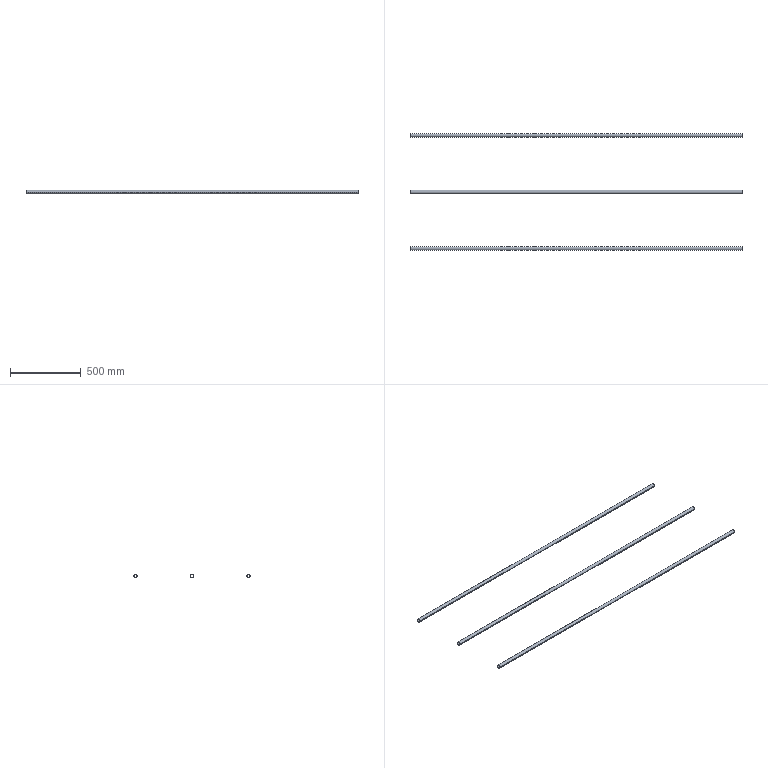Part | STEP file | E3-中转釜护栏4栏杆_Default<As Machined> | 3 solids | 18 faces | box 2348 x 825 x 25 mm | volume 780061 mm3 | cylinder 12 | plane 6 | commonest cylinder face diameters 22 x6 25 x6
STEP:
#1=CARTESIAN_POINT('',(0.,0.,0.));
#2=DIRECTION('',(0.,0.,1.));
#3=DIRECTION('',(1.,0.,0.));
#4=AXIS2_PLACEMENT_3D('',#1,#2,#3);
#5=CARTESIAN_POINT('',(1174.,787.5,0.));
#6=VERTEX_POINT('',#5);
#7=CARTESIAN_POINT('',(1174.,812.5,0.));
#8=VERTEX_POINT('',#7);
#9=CARTESIAN_POINT('',(1174.,800.,0.));
#10=DIRECTION('',(-1.,0.,0.));
#11=DIRECTION('',(0.,1.,0.));
#12=AXIS2_PLACEMENT_3D('',#9,#10,#11);
#13=CIRCLE('',#12,12.5);
#14=CARTESIAN_POINT('',(1174.,800.,0.));
#15=DIRECTION('',(-1.,0.,0.));
#16=DIRECTION('',(0.,-1.,0.));
#17=AXIS2_PLACEMENT_3D('',#14,#15,#16);
#18=CYLINDRICAL_SURFACE('',#17,12.5);
#19=CARTESIAN_POINT('',(-3.142,0.));
#20=DIRECTION('',(1.,0.));
#21=VECTOR('',#20,1.);
#22=LINE('',#19,#21);
#23=(GEOMETRIC_REPRESENTATION_CONTEXT(2)PARAMETRIC_REPRESENTATION_CONTEXT()REPRESENTATION_CONTEXT('',''));
#24=DEFINITIONAL_REPRESENTATION('',(#22),#23);
#25=PCURVE('',#18,#24);
#26=CARTESIAN_POINT('',(1174.,800.,0.));
#27=DIRECTION('',(1.,0.,0.));
#28=DIRECTION('',(0.,1.,0.));
#29=AXIS2_PLACEMENT_3D('',#26,#27,#28);
#30=PLANE('',#29);
#31=CARTESIAN_POINT('',(12.5,0.));
#32=CARTESIAN_POINT('',(12.5,-21.651));
#33=CARTESIAN_POINT('',(-6.25,-10.825));
#34=CARTESIAN_POINT('',(-25.,0.));
#35=CARTESIAN_POINT('',(-6.25,10.825));
#36=CARTESIAN_POINT('',(12.5,21.651));
#37=CARTESIAN_POINT('',(12.5,0.));
#38=(BOUNDED_CURVE()B_SPLINE_CURVE(2,(#31,#32,#33,#34,#35,#36,#37),.UNSPECIFIED.,.T.,.F.)B_SPLINE_CURVE_WITH_KNOTS((1,2,2,2,2,1),(-2.094,0.,2.094,4.189,6.283,8.378),.UNSPECIFIED.)CURVE()GEOMETRIC_REPRESENTATION_ITEM()RATIONAL_B_SPLINE_CURVE((1.,0.5,1.,0.5,1.,0.5,1.))REPRESENTATION_ITEM(''));
#39=(GEOMETRIC_REPRESENTATION_CONTEXT(2)PARAMETRIC_REPRESENTATION_CONTEXT()REPRESENTATION_CONTEXT('',''));
#40=DEFINITIONAL_REPRESENTATION('',(#38),#39);
#41=PCURVE('',#30,#40);
#42=SURFACE_CURVE('',#13,(#25,#41),.PCURVE_S1.);
#43=EDGE_CURVE('',#6,#8,#42,.T.);
#44=ORIENTED_EDGE('',*,*,#43,.T.);
#45=CARTESIAN_POINT('',(-1174.,812.5,0.));
#46=VERTEX_POINT('',#45);
#47=CARTESIAN_POINT('',(1174.,812.5,0.));
#48=DIRECTION('',(-1.,0.,0.));
#49=VECTOR('',#48,1.);
#50=LINE('',#47,#49);
#51=CARTESIAN_POINT('',(3.142,0.));
#52=DIRECTION('',(0.,1.));
#53=VECTOR('',#52,1.);
#54=LINE('',#51,#53);
#55=(GEOMETRIC_REPRESENTATION_CONTEXT(2)PARAMETRIC_REPRESENTATION_CONTEXT()REPRESENTATION_CONTEXT('',''));
#56=DEFINITIONAL_REPRESENTATION('',(#54),#55);
#57=PCURVE('',#18,#56);
#58=CARTESIAN_POINT('',(1174.,800.,0.));
#59=DIRECTION('',(-1.,0.,0.));
#60=DIRECTION('',(0.,-1.,0.));
#61=AXIS2_PLACEMENT_3D('',#58,#59,#60);
#62=CYLINDRICAL_SURFACE('',#61,12.5);
#63=CARTESIAN_POINT('',(3.142,0.));
#64=DIRECTION('',(0.,1.));
#65=VECTOR('',#64,1.);
#66=LINE('',#63,#65);
#67=(GEOMETRIC_REPRESENTATION_CONTEXT(2)PARAMETRIC_REPRESENTATION_CONTEXT()REPRESENTATION_CONTEXT('',''));
#68=DEFINITIONAL_REPRESENTATION('',(#66),#67);
#69=PCURVE('',#62,#68);
#70=SURFACE_CURVE('',#50,(#57,#69),.PCURVE_S1.);
#71=EDGE_CURVE('',#8,#46,#70,.T.);
#72=ORIENTED_EDGE('',*,*,#71,.T.);
#73=CARTESIAN_POINT('',(-1174.,787.5,0.));
#74=VERTEX_POINT('',#73);
#75=CARTESIAN_POINT('',(-1174.,800.,0.));
#76=DIRECTION('',(-1.,0.,0.));
#77=DIRECTION('',(0.,1.,0.));
#78=AXIS2_PLACEMENT_3D('',#75,#76,#77);
#79=CIRCLE('',#78,12.5);
#80=CARTESIAN_POINT('',(-3.142,2348.));
#81=DIRECTION('',(1.,0.));
#82=VECTOR('',#81,1.);
#83=LINE('',#80,#82);
#84=(GEOMETRIC_REPRESENTATION_CONTEXT(2)PARAMETRIC_REPRESENTATION_CONTEXT()REPRESENTATION_CONTEXT('',''));
#85=DEFINITIONAL_REPRESENTATION('',(#83),#84);
#86=PCURVE('',#18,#85);
#87=CARTESIAN_POINT('',(-1174.,800.,0.));
#88=DIRECTION('',(1.,0.,0.));
#89=DIRECTION('',(0.,1.,0.));
#90=AXIS2_PLACEMENT_3D('',#87,#88,#89);
#91=PLANE('',#90);
#92=CARTESIAN_POINT('',(12.5,0.));
#93=CARTESIAN_POINT('',(12.5,-21.651));
#94=CARTESIAN_POINT('',(-6.25,-10.825));
#95=CARTESIAN_POINT('',(-25.,0.));
#96=CARTESIAN_POINT('',(-6.25,10.825));
#97=CARTESIAN_POINT('',(12.5,21.651));
#98=CARTESIAN_POINT('',(12.5,0.));
#99=(BOUNDED_CURVE()B_SPLINE_CURVE(2,(#92,#93,#94,#95,#96,#97,#98),.UNSPECIFIED.,.T.,.F.)B_SPLINE_CURVE_WITH_KNOTS((1,2,2,2,2,1),(-2.094,0.,2.094,4.189,6.283,8.378),.UNSPECIFIED.)CURVE()GEOMETRIC_REPRESENTATION_ITEM()RATIONAL_B_SPLINE_CURVE((1.,0.5,1.,0.5,1.,0.5,1.))REPRESENTATION_ITEM(''));
#100=(GEOMETRIC_REPRESENTATION_CONTEXT(2)PARAMETRIC_REPRESENTATION_CONTEXT()REPRESENTATION_CONTEXT('',''));
#101=DEFINITIONAL_REPRESENTATION('',(#99),#100);
#102=PCURVE('',#91,#101);
#103=SURFACE_CURVE('',#79,(#86,#102),.PCURVE_S1.);
#104=EDGE_CURVE('',#74,#46,#103,.T.);
#105=ORIENTED_EDGE('',*,*,#104,.F.);
#106=CARTESIAN_POINT('',(1174.,787.5,0.));
#107=DIRECTION('',(-1.,0.,0.));
#108=VECTOR('',#107,1.);
#109=LINE('',#106,#108);
#110=CARTESIAN_POINT('',(0.,0.));
#111=DIRECTION('',(0.,1.));
#112=VECTOR('',#111,1.);
#113=LINE('',#110,#112);
#114=(GEOMETRIC_REPRESENTATION_CONTEXT(2)PARAMETRIC_REPRESENTATION_CONTEXT()REPRESENTATION_CONTEXT('',''));
#115=DEFINITIONAL_REPRESENTATION('',(#113),#114);
#116=PCURVE('',#18,#115);
#117=CARTESIAN_POINT('',(6.283,0.));
#118=DIRECTION('',(0.,1.));
#119=VECTOR('',#118,1.);
#120=LINE('',#117,#119);
#121=(GEOMETRIC_REPRESENTATION_CONTEXT(2)PARAMETRIC_REPRESENTATION_CONTEXT()REPRESENTATION_CONTEXT('',''));
#122=DEFINITIONAL_REPRESENTATION('',(#120),#121);
#123=PCURVE('',#62,#122);
#124=SURFACE_CURVE('',#109,(#116,#123),.PCURVE_S1.);
#125=EDGE_CURVE('',#6,#74,#124,.T.);
#126=ORIENTED_EDGE('',*,*,#125,.F.);
#127=EDGE_LOOP('',(#44,#72,#105,#126));
#128=FACE_BOUND('',#127,.T.);
#129=ADVANCED_FACE('',(#128),#18,.T.);
#130=CARTESIAN_POINT('',(1174.,789.,0.));
#131=VERTEX_POINT('',#130);
#132=CARTESIAN_POINT('',(-1174.,789.,0.));
#133=VERTEX_POINT('',#132);
#134=CARTESIAN_POINT('',(1174.,789.,0.));
#135=DIRECTION('',(-1.,0.,0.));
#136=VECTOR('',#135,1.);
#137=LINE('',#134,#136);
#138=CARTESIAN_POINT('',(1174.,800.,0.));
#139=DIRECTION('',(-1.,0.,0.));
#140=DIRECTION('',(0.,-1.,0.));
#141=AXIS2_PLACEMENT_3D('',#138,#139,#140);
#142=CYLINDRICAL_SURFACE('',#141,11.);
#143=CARTESIAN_POINT('',(6.283,0.));
#144=DIRECTION('',(0.,1.));
#145=VECTOR('',#144,1.);
#146=LINE('',#143,#145);
#147=(GEOMETRIC_REPRESENTATION_CONTEXT(2)PARAMETRIC_REPRESENTATION_CONTEXT()REPRESENTATION_CONTEXT('',''));
#148=DEFINITIONAL_REPRESENTATION('',(#146),#147);
#149=PCURVE('',#142,#148);
#150=CARTESIAN_POINT('',(1174.,800.,0.));
#151=DIRECTION('',(-1.,0.,0.));
#152=DIRECTION('',(0.,-1.,0.));
#153=AXIS2_PLACEMENT_3D('',#150,#151,#152);
#154=CYLINDRICAL_SURFACE('',#153,11.);
#155=CARTESIAN_POINT('',(0.,0.));
#156=DIRECTION('',(0.,1.));
#157=VECTOR('',#156,1.);
#158=LINE('',#155,#157);
#159=(GEOMETRIC_REPRESENTATION_CONTEXT(2)PARAMETRIC_REPRESENTATION_CONTEXT()REPRESENTATION_CONTEXT('',''));
#160=DEFINITIONAL_REPRESENTATION('',(#158),#159);
#161=PCURVE('',#154,#160);
#162=SURFACE_CURVE('',#137,(#149,#161),.PCURVE_S1.);
#163=EDGE_CURVE('',#131,#133,#162,.T.);
#164=ORIENTED_EDGE('',*,*,#163,.T.);
#165=CARTESIAN_POINT('',(-1174.,811.,0.));
#166=VERTEX_POINT('',#165);
#167=CARTESIAN_POINT('',(-1174.,800.,0.));
#168=DIRECTION('',(-1.,0.,0.));
#169=DIRECTION('',(0.,1.,0.));
#170=AXIS2_PLACEMENT_3D('',#167,#168,#169);
#171=CIRCLE('',#170,11.);
#172=CARTESIAN_POINT('',(3.142,2348.));
#173=DIRECTION('',(1.,0.));
#174=VECTOR('',#173,1.);
#175=LINE('',#172,#174);
#176=(GEOMETRIC_REPRESENTATION_CONTEXT(2)PARAMETRIC_REPRESENTATION_CONTEXT()REPRESENTATION_CONTEXT('',''));
#177=DEFINITIONAL_REPRESENTATION('',(#175),#176);
#178=PCURVE('',#142,#177);
#179=CARTESIAN_POINT('',(11.,0.));
#180=CARTESIAN_POINT('',(11.,-19.053));
#181=CARTESIAN_POINT('',(-5.5,-9.526));
#182=CARTESIAN_POINT('',(-22.,0.));
#183=CARTESIAN_POINT('',(-5.5,9.526));
#184=CARTESIAN_POINT('',(11.,19.053));
#185=CARTESIAN_POINT('',(11.,0.));
#186=(BOUNDED_CURVE()B_SPLINE_CURVE(2,(#179,#180,#181,#182,#183,#184,#185),.UNSPECIFIED.,.T.,.F.)B_SPLINE_CURVE_WITH_KNOTS((1,2,2,2,2,1),(-2.094,0.,2.094,4.189,6.283,8.378),.UNSPECIFIED.)CURVE()GEOMETRIC_REPRESENTATION_ITEM()RATIONAL_B_SPLINE_CURVE((1.,0.5,1.,0.5,1.,0.5,1.))REPRESENTATION_ITEM(''));
#187=(GEOMETRIC_REPRESENTATION_CONTEXT(2)PARAMETRIC_REPRESENTATION_CONTEXT()REPRESENTATION_CONTEXT('',''));
#188=DEFINITIONAL_REPRESENTATION('',(#186),#187);
#189=PCURVE('',#91,#188);
#190=SURFACE_CURVE('',#171,(#178,#189),.PCURVE_S1.);
#191=EDGE_CURVE('',#166,#133,#190,.T.);
#192=ORIENTED_EDGE('',*,*,#191,.F.);
#193=CARTESIAN_POINT('',(1174.,811.,0.));
#194=VERTEX_POINT('',#193);
#195=CARTESIAN_POINT('',(1174.,811.,0.));
#196=DIRECTION('',(-1.,0.,0.));
#197=VECTOR('',#196,1.);
#198=LINE('',#195,#197);
#199=CARTESIAN_POINT('',(3.142,0.));
#200=DIRECTION('',(0.,1.));
#201=VECTOR('',#200,1.);
#202=LINE('',#199,#201);
#203=(GEOMETRIC_REPRESENTATION_CONTEXT(2)PARAMETRIC_REPRESENTATION_CONTEXT()REPRESENTATION_CONTEXT('',''));
#204=DEFINITIONAL_REPRESENTATION('',(#202),#203);
#205=PCURVE('',#142,#204);
#206=CARTESIAN_POINT('',(3.142,0.));
#207=DIRECTION('',(0.,1.));
#208=VECTOR('',#207,1.);
#209=LINE('',#206,#208);
#210=(GEOMETRIC_REPRESENTATION_CONTEXT(2)PARAMETRIC_REPRESENTATION_CONTEXT()REPRESENTATION_CONTEXT('',''));
#211=DEFINITIONAL_REPRESENTATION('',(#209),#210);
#212=PCURVE('',#154,#211);
#213=SURFACE_CURVE('',#198,(#205,#212),.PCURVE_S1.);
#214=EDGE_CURVE('',#194,#166,#213,.T.);
#215=ORIENTED_EDGE('',*,*,#214,.F.);
#216=CARTESIAN_POINT('',(1174.,800.,0.));
#217=DIRECTION('',(-1.,0.,0.));
#218=DIRECTION('',(0.,1.,0.));
#219=AXIS2_PLACEMENT_3D('',#216,#217,#218);
#220=CIRCLE('',#219,11.);
#221=CARTESIAN_POINT('',(3.142,0.));
#222=DIRECTION('',(1.,0.));
#223=VECTOR('',#222,1.);
#224=LINE('',#221,#223);
#225=(GEOMETRIC_REPRESENTATION_CONTEXT(2)PARAMETRIC_REPRESENTATION_CONTEXT()REPRESENTATION_CONTEXT('',''));
#226=DEFINITIONAL_REPRESENTATION('',(#224),#225);
#227=PCURVE('',#142,#226);
#228=CARTESIAN_POINT('',(11.,0.));
#229=CARTESIAN_POINT('',(11.,-19.053));
#230=CARTESIAN_POINT('',(-5.5,-9.526));
#231=CARTESIAN_POINT('',(-22.,0.));
#232=CARTESIAN_POINT('',(-5.5,9.526));
#233=CARTESIAN_POINT('',(11.,19.053));
#234=CARTESIAN_POINT('',(11.,0.));
#235=(BOUNDED_CURVE()B_SPLINE_CURVE(2,(#228,#229,#230,#231,#232,#233,#234),.UNSPECIFIED.,.T.,.F.)B_SPLINE_CURVE_WITH_KNOTS((1,2,2,2,2,1),(-2.094,0.,2.094,4.189,6.283,8.378),.UNSPECIFIED.)CURVE()GEOMETRIC_REPRESENTATION_ITEM()RATIONAL_B_SPLINE_CURVE((1.,0.5,1.,0.5,1.,0.5,1.))REPRESENTATION_ITEM(''));
#236=(GEOMETRIC_REPRESENTATION_CONTEXT(2)PARAMETRIC_REPRESENTATION_CONTEXT()REPRESENTATION_CONTEXT('',''));
#237=DEFINITIONAL_REPRESENTATION('',(#235),#236);
#238=PCURVE('',#30,#237);
#239=SURFACE_CURVE('',#220,(#227,#238),.PCURVE_S1.);
#240=EDGE_CURVE('',#194,#131,#239,.T.);
#241=ORIENTED_EDGE('',*,*,#240,.T.);
#242=EDGE_LOOP('',(#164,#192,#215,#241));
#243=FACE_BOUND('',#242,.F.);
#244=ADVANCED_FACE('',(#243),#142,.F.);
#245=CARTESIAN_POINT('',(-1174.,800.,0.));
#246=DIRECTION('',(-1.,0.,0.));
#247=DIRECTION('',(0.,1.,0.));
#248=AXIS2_PLACEMENT_3D('',#245,#246,#247);
#249=CIRCLE('',#248,11.);
#250=CARTESIAN_POINT('',(-3.142,2348.));
#251=DIRECTION('',(1.,0.));
#252=VECTOR('',#251,1.);
#253=LINE('',#250,#252);
#254=(GEOMETRIC_REPRESENTATION_CONTEXT(2)PARAMETRIC_REPRESENTATION_CONTEXT()REPRESENTATION_CONTEXT('',''));
#255=DEFINITIONAL_REPRESENTATION('',(#253),#254);
#256=PCURVE('',#154,#255);
#257=CARTESIAN_POINT('',(11.,0.));
#258=CARTESIAN_POINT('',(11.,-19.053));
#259=CARTESIAN_POINT('',(-5.5,-9.526));
#260=CARTESIAN_POINT('',(-22.,0.));
#261=CARTESIAN_POINT('',(-5.5,9.526));
#262=CARTESIAN_POINT('',(11.,19.053));
#263=CARTESIAN_POINT('',(11.,0.));
#264=(BOUNDED_CURVE()B_SPLINE_CURVE(2,(#257,#258,#259,#260,#261,#262,#263),.UNSPECIFIED.,.T.,.F.)B_SPLINE_CURVE_WITH_KNOTS((1,2,2,2,2,1),(-2.094,0.,2.094,4.189,6.283,8.378),.UNSPECIFIED.)CURVE()GEOMETRIC_REPRESENTATION_ITEM()RATIONAL_B_SPLINE_CURVE((1.,0.5,1.,0.5,1.,0.5,1.))REPRESENTATION_ITEM(''));
#265=(GEOMETRIC_REPRESENTATION_CONTEXT(2)PARAMETRIC_REPRESENTATION_CONTEXT()REPRESENTATION_CONTEXT('',''));
#266=DEFINITIONAL_REPRESENTATION('',(#264),#265);
#267=PCURVE('',#91,#266);
#268=SURFACE_CURVE('',#249,(#256,#267),.PCURVE_S1.);
#269=EDGE_CURVE('',#133,#166,#268,.T.);
#270=ORIENTED_EDGE('',*,*,#269,.F.);
#271=ORIENTED_EDGE('',*,*,#163,.F.);
#272=CARTESIAN_POINT('',(1174.,800.,0.));
#273=DIRECTION('',(-1.,0.,0.));
#274=DIRECTION('',(0.,1.,0.));
#275=AXIS2_PLACEMENT_3D('',#272,#273,#274);
#276=CIRCLE('',#275,11.);
#277=CARTESIAN_POINT('',(-3.142,0.));
#278=DIRECTION('',(1.,0.));
#279=VECTOR('',#278,1.);
#280=LINE('',#277,#279);
#281=(GEOMETRIC_REPRESENTATION_CONTEXT(2)PARAMETRIC_REPRESENTATION_CONTEXT()REPRESENTATION_CONTEXT('',''));
#282=DEFINITIONAL_REPRESENTATION('',(#280),#281);
#283=PCURVE('',#154,#282);
#284=CARTESIAN_POINT('',(11.,0.));
#285=CARTESIAN_POINT('',(11.,-19.053));
#286=CARTESIAN_POINT('',(-5.5,-9.526));
#287=CARTESIAN_POINT('',(-22.,0.));
#288=CARTESIAN_POINT('',(-5.5,9.526));
#289=CARTESIAN_POINT('',(11.,19.053));
#290=CARTESIAN_POINT('',(11.,0.));
#291=(BOUNDED_CURVE()B_SPLINE_CURVE(2,(#284,#285,#286,#287,#288,#289,#290),.UNSPECIFIED.,.T.,.F.)B_SPLINE_CURVE_WITH_KNOTS((1,2,2,2,2,1),(-2.094,0.,2.094,4.189,6.283,8.378),.UNSPECIFIED.)CURVE()GEOMETRIC_REPRESENTATION_ITEM()RATIONAL_B_SPLINE_CURVE((1.,0.5,1.,0.5,1.,0.5,1.))REPRESENTATION_ITEM(''));
#292=(GEOMETRIC_REPRESENTATION_CONTEXT(2)PARAMETRIC_REPRESENTATION_CONTEXT()REPRESENTATION_CONTEXT('',''));
#293=DEFINITIONAL_REPRESENTATION('',(#291),#292);
#294=PCURVE('',#30,#293);
#295=SURFACE_CURVE('',#276,(#283,#294),.PCURVE_S1.);
#296=EDGE_CURVE('',#131,#194,#295,.T.);
#297=ORIENTED_EDGE('',*,*,#296,.T.);
#298=ORIENTED_EDGE('',*,*,#214,.T.);
#299=EDGE_LOOP('',(#270,#271,#297,#298));
#300=FACE_BOUND('',#299,.F.);
#301=ADVANCED_FACE('',(#300),#154,.F.);
#302=ORIENTED_EDGE('',*,*,#71,.F.);
#303=CARTESIAN_POINT('',(1174.,800.,0.));
#304=DIRECTION('',(-1.,0.,0.));
#305=DIRECTION('',(0.,1.,0.));
#306=AXIS2_PLACEMENT_3D('',#303,#304,#305);
#307=CIRCLE('',#306,12.5);
#308=CARTESIAN_POINT('',(3.142,0.));
#309=DIRECTION('',(1.,0.));
#310=VECTOR('',#309,1.);
#311=LINE('',#308,#310);
#312=(GEOMETRIC_REPRESENTATION_CONTEXT(2)PARAMETRIC_REPRESENTATION_CONTEXT()REPRESENTATION_CONTEXT('',''));
#313=DEFINITIONAL_REPRESENTATION('',(#311),#312);
#314=PCURVE('',#62,#313);
#315=CARTESIAN_POINT('',(12.5,0.));
#316=CARTESIAN_POINT('',(12.5,-21.651));
#317=CARTESIAN_POINT('',(-6.25,-10.825));
#318=CARTESIAN_POINT('',(-25.,0.));
#319=CARTESIAN_POINT('',(-6.25,10.825));
#320=CARTESIAN_POINT('',(12.5,21.651));
#321=CARTESIAN_POINT('',(12.5,0.));
#322=(BOUNDED_CURVE()B_SPLINE_CURVE(2,(#315,#316,#317,#318,#319,#320,#321),.UNSPECIFIED.,.T.,.F.)B_SPLINE_CURVE_WITH_KNOTS((1,2,2,2,2,1),(-2.094,0.,2.094,4.189,6.283,8.378),.UNSPECIFIED.)CURVE()GEOMETRIC_REPRESENTATION_ITEM()RATIONAL_B_SPLINE_CURVE((1.,0.5,1.,0.5,1.,0.5,1.))REPRESENTATION_ITEM(''));
#323=(GEOMETRIC_REPRESENTATION_CONTEXT(2)PARAMETRIC_REPRESENTATION_CONTEXT()REPRESENTATION_CONTEXT('',''));
#324=DEFINITIONAL_REPRESENTATION('',(#322),#323);
#325=PCURVE('',#30,#324);
#326=SURFACE_CURVE('',#307,(#314,#325),.PCURVE_S1.);
#327=EDGE_CURVE('',#8,#6,#326,.T.);
#328=ORIENTED_EDGE('',*,*,#327,.T.);
#329=ORIENTED_EDGE('',*,*,#125,.T.);
#330=CARTESIAN_POINT('',(-1174.,800.,0.));
#331=DIRECTION('',(-1.,0.,0.));
#332=DIRECTION('',(0.,1.,0.));
#333=AXIS2_PLACEMENT_3D('',#330,#331,#332);
#334=CIRCLE('',#333,12.5);
#335=CARTESIAN_POINT('',(3.142,2348.));
#336=DIRECTION('',(1.,0.));
#337=VECTOR('',#336,1.);
#338=LINE('',#335,#337);
#339=(GEOMETRIC_REPRESENTATION_CONTEXT(2)PARAMETRIC_REPRESENTATION_CONTEXT()REPRESENTATION_CONTEXT('',''));
#340=DEFINITIONAL_REPRESENTATION('',(#338),#339);
#341=PCURVE('',#62,#340);
#342=CARTESIAN_POINT('',(12.5,0.));
#343=CARTESIAN_POINT('',(12.5,-21.651));
#344=CARTESIAN_POINT('',(-6.25,-10.825));
#345=CARTESIAN_POINT('',(-25.,0.));
#346=CARTESIAN_POINT('',(-6.25,10.825));
#347=CARTESIAN_POINT('',(12.5,21.651));
#348=CARTESIAN_POINT('',(12.5,0.));
#349=(BOUNDED_CURVE()B_SPLINE_CURVE(2,(#342,#343,#344,#345,#346,#347,#348),.UNSPECIFIED.,.T.,.F.)B_SPLINE_CURVE_WITH_KNOTS((1,2,2,2,2,1),(-2.094,0.,2.094,4.189,6.283,8.378),.UNSPECIFIED.)CURVE()GEOMETRIC_REPRESENTATION_ITEM()RATIONAL_B_SPLINE_CURVE((1.,0.5,1.,0.5,1.,0.5,1.))REPRESENTATION_ITEM(''));
#350=(GEOMETRIC_REPRESENTATION_CONTEXT(2)PARAMETRIC_REPRESENTATION_CONTEXT()REPRESENTATION_CONTEXT('',''));
#351=DEFINITIONAL_REPRESENTATION('',(#349),#350);
#352=PCURVE('',#91,#351);
#353=SURFACE_CURVE('',#334,(#341,#352),.PCURVE_S1.);
#354=EDGE_CURVE('',#46,#74,#353,.T.);
#355=ORIENTED_EDGE('',*,*,#354,.F.);
#356=EDGE_LOOP('',(#302,#328,#329,#355));
#357=FACE_BOUND('',#356,.T.);
#358=ADVANCED_FACE('',(#357),#62,.T.);
#359=ORIENTED_EDGE('',*,*,#296,.T.);
#360=ORIENTED_EDGE('',*,*,#240,.T.);
#361=EDGE_LOOP('',(#359,#360));
#362=FACE_BOUND('',#361,.T.);
#363=ORIENTED_EDGE('',*,*,#43,.F.);
#364=ORIENTED_EDGE('',*,*,#327,.F.);
#365=EDGE_LOOP('',(#363,#364));
#366=FACE_BOUND('',#365,.T.);
#367=ADVANCED_FACE('',(#362,#366),#30,.T.);
#368=ORIENTED_EDGE('',*,*,#269,.F.);
#369=ORIENTED_EDGE('',*,*,#191,.F.);
#370=EDGE_LOOP('',(#368,#369));
#371=FACE_BOUND('',#370,.T.);
#372=ORIENTED_EDGE('',*,*,#104,.T.);
#373=ORIENTED_EDGE('',*,*,#354,.T.);
#374=EDGE_LOOP('',(#372,#373));
#375=FACE_BOUND('',#374,.T.);
#376=ADVANCED_FACE('',(#371,#375),#91,.F.);
#377=CLOSED_SHELL('',(#129,#244,#301,#358,#367,#376));
#378=MANIFOLD_SOLID_BREP('',#377);
#379=CARTESIAN_POINT('',(1174.,-12.5,0.));
#380=VERTEX_POINT('',#379);
#381=CARTESIAN_POINT('',(1174.,12.5,0.));
#382=VERTEX_POINT('',#381);
#383=CARTESIAN_POINT('',(1174.,0.,0.));
#384=DIRECTION('',(-1.,0.,0.));
#385=DIRECTION('',(0.,1.,0.));
#386=AXIS2_PLACEMENT_3D('',#383,#384,#385);
#387=CIRCLE('',#386,12.5);
#388=CARTESIAN_POINT('',(1174.,0.,0.));
#389=DIRECTION('',(-1.,0.,0.));
#390=DIRECTION('',(0.,-1.,0.));
#391=AXIS2_PLACEMENT_3D('',#388,#389,#390);
#392=CYLINDRICAL_SURFACE('',#391,12.5);
#393=CARTESIAN_POINT('',(-3.142,0.));
#394=DIRECTION('',(1.,0.));
#395=VECTOR('',#394,1.);
#396=LINE('',#393,#395);
#397=(GEOMETRIC_REPRESENTATION_CONTEXT(2)PARAMETRIC_REPRESENTATION_CONTEXT()REPRESENTATION_CONTEXT('',''));
#398=DEFINITIONAL_REPRESENTATION('',(#396),#397);
#399=PCURVE('',#392,#398);
#400=CARTESIAN_POINT('',(1174.,0.,0.));
#401=DIRECTION('',(1.,0.,0.));
#402=DIRECTION('',(0.,1.,0.));
#403=AXIS2_PLACEMENT_3D('',#400,#401,#402);
#404=PLANE('',#403);
#405=CARTESIAN_POINT('',(12.5,0.));
#406=CARTESIAN_POINT('',(12.5,-21.651));
#407=CARTESIAN_POINT('',(-6.25,-10.825));
#408=CARTESIAN_POINT('',(-25.,0.));
#409=CARTESIAN_POINT('',(-6.25,10.825));
#410=CARTESIAN_POINT('',(12.5,21.651));
#411=CARTESIAN_POINT('',(12.5,0.));
#412=(BOUNDED_CURVE()B_SPLINE_CURVE(2,(#405,#406,#407,#408,#409,#410,#411),.UNSPECIFIED.,.T.,.F.)B_SPLINE_CURVE_WITH_KNOTS((1,2,2,2,2,1),(-2.094,0.,2.094,4.189,6.283,8.378),.UNSPECIFIED.)CURVE()GEOMETRIC_REPRESENTATION_ITEM()RATIONAL_B_SPLINE_CURVE((1.,0.5,1.,0.5,1.,0.5,1.))REPRESENTATION_ITEM(''));
#413=(GEOMETRIC_REPRESENTATION_CONTEXT(2)PARAMETRIC_REPRESENTATION_CONTEXT()REPRESENTATION_CONTEXT('',''));
#414=DEFINITIONAL_REPRESENTATION('',(#412),#413);
#415=PCURVE('',#404,#414);
#416=SURFACE_CURVE('',#387,(#399,#415),.PCURVE_S1.);
#417=EDGE_CURVE('',#380,#382,#416,.T.);
#418=ORIENTED_EDGE('',*,*,#417,.T.);
#419=CARTESIAN_POINT('',(-1174.,12.5,0.));
#420=VERTEX_POINT('',#419);
#421=CARTESIAN_POINT('',(1174.,12.5,0.));
#422=DIRECTION('',(-1.,0.,0.));
#423=VECTOR('',#422,1.);
#424=LINE('',#421,#423);
#425=CARTESIAN_POINT('',(3.142,0.));
#426=DIRECTION('',(0.,1.));
#427=VECTOR('',#426,1.);
#428=LINE('',#425,#427);
#429=(GEOMETRIC_REPRESENTATION_CONTEXT(2)PARAMETRIC_REPRESENTATION_CONTEXT()REPRESENTATION_CONTEXT('',''));
#430=DEFINITIONAL_REPRESENTATION('',(#428),#429);
#431=PCURVE('',#392,#430);
#432=CARTESIAN_POINT('',(1174.,0.,0.));
#433=DIRECTION('',(-1.,0.,0.));
#434=DIRECTION('',(0.,-1.,0.));
#435=AXIS2_PLACEMENT_3D('',#432,#433,#434);
#436=CYLINDRICAL_SURFACE('',#435,12.5);
#437=CARTESIAN_POINT('',(3.142,0.));
#438=DIRECTION('',(0.,1.));
#439=VECTOR('',#438,1.);
#440=LINE('',#437,#439);
#441=(GEOMETRIC_REPRESENTATION_CONTEXT(2)PARAMETRIC_REPRESENTATION_CONTEXT()REPRESENTATION_CONTEXT('',''));
#442=DEFINITIONAL_REPRESENTATION('',(#440),#441);
#443=PCURVE('',#436,#442);
#444=SURFACE_CURVE('',#424,(#431,#443),.PCURVE_S1.);
#445=EDGE_CURVE('',#382,#420,#444,.T.);
#446=ORIENTED_EDGE('',*,*,#445,.T.);
#447=CARTESIAN_POINT('',(-1174.,-12.5,0.));
#448=VERTEX_POINT('',#447);
#449=CARTESIAN_POINT('',(-1174.,0.,0.));
#450=DIRECTION('',(-1.,0.,0.));
#451=DIRECTION('',(0.,1.,0.));
#452=AXIS2_PLACEMENT_3D('',#449,#450,#451);
#453=CIRCLE('',#452,12.5);
#454=CARTESIAN_POINT('',(-3.142,2348.));
#455=DIRECTION('',(1.,0.));
#456=VECTOR('',#455,1.);
#457=LINE('',#454,#456);
#458=(GEOMETRIC_REPRESENTATION_CONTEXT(2)PARAMETRIC_REPRESENTATION_CONTEXT()REPRESENTATION_CONTEXT('',''));
#459=DEFINITIONAL_REPRESENTATION('',(#457),#458);
#460=PCURVE('',#392,#459);
#461=CARTESIAN_POINT('',(-1174.,0.,0.));
#462=DIRECTION('',(1.,0.,0.));
#463=DIRECTION('',(0.,1.,0.));
#464=AXIS2_PLACEMENT_3D('',#461,#462,#463);
#465=PLANE('',#464);
#466=CARTESIAN_POINT('',(12.5,0.));
#467=CARTESIAN_POINT('',(12.5,-21.651));
#468=CARTESIAN_POINT('',(-6.25,-10.825));
#469=CARTESIAN_POINT('',(-25.,0.));
#470=CARTESIAN_POINT('',(-6.25,10.825));
#471=CARTESIAN_POINT('',(12.5,21.651));
#472=CARTESIAN_POINT('',(12.5,0.));
#473=(BOUNDED_CURVE()B_SPLINE_CURVE(2,(#466,#467,#468,#469,#470,#471,#472),.UNSPECIFIED.,.T.,.F.)B_SPLINE_CURVE_WITH_KNOTS((1,2,2,2,2,1),(-2.094,0.,2.094,4.189,6.283,8.378),.UNSPECIFIED.)CURVE()GEOMETRIC_REPRESENTATION_ITEM()RATIONAL_B_SPLINE_CURVE((1.,0.5,1.,0.5,1.,0.5,1.))REPRESENTATION_ITEM(''));
#474=(GEOMETRIC_REPRESENTATION_CONTEXT(2)PARAMETRIC_REPRESENTATION_CONTEXT()REPRESENTATION_CONTEXT('',''));
#475=DEFINITIONAL_REPRESENTATION('',(#473),#474);
#476=PCURVE('',#465,#475);
#477=SURFACE_CURVE('',#453,(#460,#476),.PCURVE_S1.);
#478=EDGE_CURVE('',#448,#420,#477,.T.);
#479=ORIENTED_EDGE('',*,*,#478,.F.);
#480=CARTESIAN_POINT('',(1174.,-12.5,0.));
#481=DIRECTION('',(-1.,0.,0.));
#482=VECTOR('',#481,1.);
#483=LINE('',#480,#482);
#484=CARTESIAN_POINT('',(0.,0.));
#485=DIRECTION('',(0.,1.));
#486=VECTOR('',#485,1.);
#487=LINE('',#484,#486);
#488=(GEOMETRIC_REPRESENTATION_CONTEXT(2)PARAMETRIC_REPRESENTATION_CONTEXT()REPRESENTATION_CONTEXT('',''));
#489=DEFINITIONAL_REPRESENTATION('',(#487),#488);
#490=PCURVE('',#392,#489);
#491=CARTESIAN_POINT('',(6.283,0.));
#492=DIRECTION('',(0.,1.));
#493=VECTOR('',#492,1.);
#494=LINE('',#491,#493);
#495=(GEOMETRIC_REPRESENTATION_CONTEXT(2)PARAMETRIC_REPRESENTATION_CONTEXT()REPRESENTATION_CONTEXT('',''));
#496=DEFINITIONAL_REPRESENTATION('',(#494),#495);
#497=PCURVE('',#436,#496);
#498=SURFACE_CURVE('',#483,(#490,#497),.PCURVE_S1.);
#499=EDGE_CURVE('',#380,#448,#498,.T.);
#500=ORIENTED_EDGE('',*,*,#499,.F.);
#501=EDGE_LOOP('',(#418,#446,#479,#500));
#502=FACE_BOUND('',#501,.T.);
#503=ADVANCED_FACE('',(#502),#392,.T.);
#504=CARTESIAN_POINT('',(1174.,-11.,0.));
#505=VERTEX_POINT('',#504);
#506=CARTESIAN_POINT('',(-1174.,-11.,0.));
#507=VERTEX_POINT('',#506);
#508=CARTESIAN_POINT('',(1174.,-11.,0.));
#509=DIRECTION('',(-1.,0.,0.));
#510=VECTOR('',#509,1.);
#511=LINE('',#508,#510);
#512=CARTESIAN_POINT('',(1174.,0.,0.));
#513=DIRECTION('',(-1.,0.,0.));
#514=DIRECTION('',(0.,-1.,0.));
#515=AXIS2_PLACEMENT_3D('',#512,#513,#514);
#516=CYLINDRICAL_SURFACE('',#515,11.);
#517=CARTESIAN_POINT('',(6.283,0.));
#518=DIRECTION('',(0.,1.));
#519=VECTOR('',#518,1.);
#520=LINE('',#517,#519);
#521=(GEOMETRIC_REPRESENTATION_CONTEXT(2)PARAMETRIC_REPRESENTATION_CONTEXT()REPRESENTATION_CONTEXT('',''));
#522=DEFINITIONAL_REPRESENTATION('',(#520),#521);
#523=PCURVE('',#516,#522);
#524=CARTESIAN_POINT('',(1174.,0.,0.));
#525=DIRECTION('',(-1.,0.,0.));
#526=DIRECTION('',(0.,-1.,0.));
#527=AXIS2_PLACEMENT_3D('',#524,#525,#526);
#528=CYLINDRICAL_SURFACE('',#527,11.);
#529=CARTESIAN_POINT('',(0.,0.));
#530=DIRECTION('',(0.,1.));
#531=VECTOR('',#530,1.);
#532=LINE('',#529,#531);
#533=(GEOMETRIC_REPRESENTATION_CONTEXT(2)PARAMETRIC_REPRESENTATION_CONTEXT()REPRESENTATION_CONTEXT('',''));
#534=DEFINITIONAL_REPRESENTATION('',(#532),#533);
#535=PCURVE('',#528,#534);
#536=SURFACE_CURVE('',#511,(#523,#535),.PCURVE_S1.);
#537=EDGE_CURVE('',#505,#507,#536,.T.);
#538=ORIENTED_EDGE('',*,*,#537,.T.);
#539=CARTESIAN_POINT('',(-1174.,11.,0.));
#540=VERTEX_POINT('',#539);
#541=CARTESIAN_POINT('',(-1174.,0.,0.));
#542=DIRECTION('',(-1.,0.,0.));
#543=DIRECTION('',(0.,1.,0.));
#544=AXIS2_PLACEMENT_3D('',#541,#542,#543);
#545=CIRCLE('',#544,11.);
#546=CARTESIAN_POINT('',(3.142,2348.));
#547=DIRECTION('',(1.,0.));
#548=VECTOR('',#547,1.);
#549=LINE('',#546,#548);
#550=(GEOMETRIC_REPRESENTATION_CONTEXT(2)PARAMETRIC_REPRESENTATION_CONTEXT()REPRESENTATION_CONTEXT('',''));
#551=DEFINITIONAL_REPRESENTATION('',(#549),#550);
#552=PCURVE('',#516,#551);
#553=CARTESIAN_POINT('',(11.,0.));
#554=CARTESIAN_POINT('',(11.,-19.053));
#555=CARTESIAN_POINT('',(-5.5,-9.526));
#556=CARTESIAN_POINT('',(-22.,0.));
#557=CARTESIAN_POINT('',(-5.5,9.526));
#558=CARTESIAN_POINT('',(11.,19.053));
#559=CARTESIAN_POINT('',(11.,0.));
#560=(BOUNDED_CURVE()B_SPLINE_CURVE(2,(#553,#554,#555,#556,#557,#558,#559),.UNSPECIFIED.,.T.,.F.)B_SPLINE_CURVE_WITH_KNOTS((1,2,2,2,2,1),(-2.094,0.,2.094,4.189,6.283,8.378),.UNSPECIFIED.)CURVE()GEOMETRIC_REPRESENTATION_ITEM()RATIONAL_B_SPLINE_CURVE((1.,0.5,1.,0.5,1.,0.5,1.))REPRESENTATION_ITEM(''));
#561=(GEOMETRIC_REPRESENTATION_CONTEXT(2)PARAMETRIC_REPRESENTATION_CONTEXT()REPRESENTATION_CONTEXT('',''));
#562=DEFINITIONAL_REPRESENTATION('',(#560),#561);
#563=PCURVE('',#465,#562);
#564=SURFACE_CURVE('',#545,(#552,#563),.PCURVE_S1.);
#565=EDGE_CURVE('',#540,#507,#564,.T.);
#566=ORIENTED_EDGE('',*,*,#565,.F.);
#567=CARTESIAN_POINT('',(1174.,11.,0.));
#568=VERTEX_POINT('',#567);
#569=CARTESIAN_POINT('',(1174.,11.,0.));
#570=DIRECTION('',(-1.,0.,0.));
#571=VECTOR('',#570,1.);
#572=LINE('',#569,#571);
#573=CARTESIAN_POINT('',(3.142,0.));
#574=DIRECTION('',(0.,1.));
#575=VECTOR('',#574,1.);
#576=LINE('',#573,#575);
#577=(GEOMETRIC_REPRESENTATION_CONTEXT(2)PARAMETRIC_REPRESENTATION_CONTEXT()REPRESENTATION_CONTEXT('',''));
#578=DEFINITIONAL_REPRESENTATION('',(#576),#577);
#579=PCURVE('',#516,#578);
#580=CARTESIAN_POINT('',(3.142,0.));
#581=DIRECTION('',(0.,1.));
#582=VECTOR('',#581,1.);
#583=LINE('',#580,#582);
#584=(GEOMETRIC_REPRESENTATION_CONTEXT(2)PARAMETRIC_REPRESENTATION_CONTEXT()REPRESENTATION_CONTEXT('',''));
#585=DEFINITIONAL_REPRESENTATION('',(#583),#584);
#586=PCURVE('',#528,#585);
#587=SURFACE_CURVE('',#572,(#579,#586),.PCURVE_S1.);
#588=EDGE_CURVE('',#568,#540,#587,.T.);
#589=ORIENTED_EDGE('',*,*,#588,.F.);
#590=CARTESIAN_POINT('',(1174.,0.,0.));
#591=DIRECTION('',(-1.,0.,0.));
#592=DIRECTION('',(0.,1.,0.));
#593=AXIS2_PLACEMENT_3D('',#590,#591,#592);
#594=CIRCLE('',#593,11.);
#595=CARTESIAN_POINT('',(3.142,0.));
#596=DIRECTION('',(1.,0.));
#597=VECTOR('',#596,1.);
#598=LINE('',#595,#597);
#599=(GEOMETRIC_REPRESENTATION_CONTEXT(2)PARAMETRIC_REPRESENTATION_CONTEXT()REPRESENTATION_CONTEXT('',''));
#600=DEFINITIONAL_REPRESENTATION('',(#598),#599);
#601=PCURVE('',#516,#600);
#602=CARTESIAN_POINT('',(11.,0.));
#603=CARTESIAN_POINT('',(11.,-19.053));
#604=CARTESIAN_POINT('',(-5.5,-9.526));
#605=CARTESIAN_POINT('',(-22.,0.));
#606=CARTESIAN_POINT('',(-5.5,9.526));
#607=CARTESIAN_POINT('',(11.,19.053));
#608=CARTESIAN_POINT('',(11.,0.));
#609=(BOUNDED_CURVE()B_SPLINE_CURVE(2,(#602,#603,#604,#605,#606,#607,#608),.UNSPECIFIED.,.T.,.F.)B_SPLINE_CURVE_WITH_KNOTS((1,2,2,2,2,1),(-2.094,0.,2.094,4.189,6.283,8.378),.UNSPECIFIED.)CURVE()GEOMETRIC_REPRESENTATION_ITEM()RATIONAL_B_SPLINE_CURVE((1.,0.5,1.,0.5,1.,0.5,1.))REPRESENTATION_ITEM(''));
#610=(GEOMETRIC_REPRESENTATION_CONTEXT(2)PARAMETRIC_REPRESENTATION_CONTEXT()REPRESENTATION_CONTEXT('',''));
#611=DEFINITIONAL_REPRESENTATION('',(#609),#610);
#612=PCURVE('',#404,#611);
#613=SURFACE_CURVE('',#594,(#601,#612),.PCURVE_S1.);
#614=EDGE_CURVE('',#568,#505,#613,.T.);
#615=ORIENTED_EDGE('',*,*,#614,.T.);
#616=EDGE_LOOP('',(#538,#566,#589,#615));
#617=FACE_BOUND('',#616,.F.);
#618=ADVANCED_FACE('',(#617),#516,.F.);
#619=CARTESIAN_POINT('',(-1174.,0.,0.));
#620=DIRECTION('',(-1.,0.,0.));
#621=DIRECTION('',(0.,1.,0.));
#622=AXIS2_PLACEMENT_3D('',#619,#620,#621);
#623=CIRCLE('',#622,11.);
#624=CARTESIAN_POINT('',(-3.142,2348.));
#625=DIRECTION('',(1.,0.));
#626=VECTOR('',#625,1.);
#627=LINE('',#624,#626);
#628=(GEOMETRIC_REPRESENTATION_CONTEXT(2)PARAMETRIC_REPRESENTATION_CONTEXT()REPRESENTATION_CONTEXT('',''));
#629=DEFINITIONAL_REPRESENTATION('',(#627),#628);
#630=PCURVE('',#528,#629);
#631=CARTESIAN_POINT('',(11.,0.));
#632=CARTESIAN_POINT('',(11.,-19.053));
#633=CARTESIAN_POINT('',(-5.5,-9.526));
#634=CARTESIAN_POINT('',(-22.,0.));
#635=CARTESIAN_POINT('',(-5.5,9.526));
#636=CARTESIAN_POINT('',(11.,19.053));
#637=CARTESIAN_POINT('',(11.,0.));
#638=(BOUNDED_CURVE()B_SPLINE_CURVE(2,(#631,#632,#633,#634,#635,#636,#637),.UNSPECIFIED.,.T.,.F.)B_SPLINE_CURVE_WITH_KNOTS((1,2,2,2,2,1),(-2.094,0.,2.094,4.189,6.283,8.378),.UNSPECIFIED.)CURVE()GEOMETRIC_REPRESENTATION_ITEM()RATIONAL_B_SPLINE_CURVE((1.,0.5,1.,0.5,1.,0.5,1.))REPRESENTATION_ITEM(''));
#639=(GEOMETRIC_REPRESENTATION_CONTEXT(2)PARAMETRIC_REPRESENTATION_CONTEXT()REPRESENTATION_CONTEXT('',''));
#640=DEFINITIONAL_REPRESENTATION('',(#638),#639);
#641=PCURVE('',#465,#640);
#642=SURFACE_CURVE('',#623,(#630,#641),.PCURVE_S1.);
#643=EDGE_CURVE('',#507,#540,#642,.T.);
#644=ORIENTED_EDGE('',*,*,#643,.F.);
#645=ORIENTED_EDGE('',*,*,#537,.F.);
#646=CARTESIAN_POINT('',(1174.,0.,0.));
#647=DIRECTION('',(-1.,0.,0.));
#648=DIRECTION('',(0.,1.,0.));
#649=AXIS2_PLACEMENT_3D('',#646,#647,#648);
#650=CIRCLE('',#649,11.);
#651=CARTESIAN_POINT('',(-3.142,0.));
#652=DIRECTION('',(1.,0.));
#653=VECTOR('',#652,1.);
#654=LINE('',#651,#653);
#655=(GEOMETRIC_REPRESENTATION_CONTEXT(2)PARAMETRIC_REPRESENTATION_CONTEXT()REPRESENTATION_CONTEXT('',''));
#656=DEFINITIONAL_REPRESENTATION('',(#654),#655);
#657=PCURVE('',#528,#656);
#658=CARTESIAN_POINT('',(11.,0.));
#659=CARTESIAN_POINT('',(11.,-19.053));
#660=CARTESIAN_POINT('',(-5.5,-9.526));
#661=CARTESIAN_POINT('',(-22.,0.));
#662=CARTESIAN_POINT('',(-5.5,9.526));
#663=CARTESIAN_POINT('',(11.,19.053));
#664=CARTESIAN_POINT('',(11.,0.));
#665=(BOUNDED_CURVE()B_SPLINE_CURVE(2,(#658,#659,#660,#661,#662,#663,#664),.UNSPECIFIED.,.T.,.F.)B_SPLINE_CURVE_WITH_KNOTS((1,2,2,2,2,1),(-2.094,0.,2.094,4.189,6.283,8.378),.UNSPECIFIED.)CURVE()GEOMETRIC_REPRESENTATION_ITEM()RATIONAL_B_SPLINE_CURVE((1.,0.5,1.,0.5,1.,0.5,1.))REPRESENTATION_ITEM(''));
#666=(GEOMETRIC_REPRESENTATION_CONTEXT(2)PARAMETRIC_REPRESENTATION_CONTEXT()REPRESENTATION_CONTEXT('',''));
#667=DEFINITIONAL_REPRESENTATION('',(#665),#666);
#668=PCURVE('',#404,#667);
#669=SURFACE_CURVE('',#650,(#657,#668),.PCURVE_S1.);
#670=EDGE_CURVE('',#505,#568,#669,.T.);
#671=ORIENTED_EDGE('',*,*,#670,.T.);
#672=ORIENTED_EDGE('',*,*,#588,.T.);
#673=EDGE_LOOP('',(#644,#645,#671,#672));
#674=FACE_BOUND('',#673,.F.);
#675=ADVANCED_FACE('',(#674),#528,.F.);
#676=ORIENTED_EDGE('',*,*,#445,.F.);
#677=CARTESIAN_POINT('',(1174.,0.,0.));
#678=DIRECTION('',(-1.,0.,0.));
#679=DIRECTION('',(0.,1.,0.));
#680=AXIS2_PLACEMENT_3D('',#677,#678,#679);
#681=CIRCLE('',#680,12.5);
#682=CARTESIAN_POINT('',(3.142,0.));
#683=DIRECTION('',(1.,0.));
#684=VECTOR('',#683,1.);
#685=LINE('',#682,#684);
#686=(GEOMETRIC_REPRESENTATION_CONTEXT(2)PARAMETRIC_REPRESENTATION_CONTEXT()REPRESENTATION_CONTEXT('',''));
#687=DEFINITIONAL_REPRESENTATION('',(#685),#686);
#688=PCURVE('',#436,#687);
#689=CARTESIAN_POINT('',(12.5,0.));
#690=CARTESIAN_POINT('',(12.5,-21.651));
#691=CARTESIAN_POINT('',(-6.25,-10.825));
#692=CARTESIAN_POINT('',(-25.,0.));
#693=CARTESIAN_POINT('',(-6.25,10.825));
#694=CARTESIAN_POINT('',(12.5,21.651));
#695=CARTESIAN_POINT('',(12.5,0.));
#696=(BOUNDED_CURVE()B_SPLINE_CURVE(2,(#689,#690,#691,#692,#693,#694,#695),.UNSPECIFIED.,.T.,.F.)B_SPLINE_CURVE_WITH_KNOTS((1,2,2,2,2,1),(-2.094,0.,2.094,4.189,6.283,8.378),.UNSPECIFIED.)CURVE()GEOMETRIC_REPRESENTATION_ITEM()RATIONAL_B_SPLINE_CURVE((1.,0.5,1.,0.5,1.,0.5,1.))REPRESENTATION_ITEM(''));
#697=(GEOMETRIC_REPRESENTATION_CONTEXT(2)PARAMETRIC_REPRESENTATION_CONTEXT()REPRESENTATION_CONTEXT('',''));
#698=DEFINITIONAL_REPRESENTATION('',(#696),#697);
#699=PCURVE('',#404,#698);
#700=SURFACE_CURVE('',#681,(#688,#699),.PCURVE_S1.);
#701=EDGE_CURVE('',#382,#380,#700,.T.);
#702=ORIENTED_EDGE('',*,*,#701,.T.);
#703=ORIENTED_EDGE('',*,*,#499,.T.);
#704=CARTESIAN_POINT('',(-1174.,0.,0.));
#705=DIRECTION('',(-1.,0.,0.));
#706=DIRECTION('',(0.,1.,0.));
#707=AXIS2_PLACEMENT_3D('',#704,#705,#706);
#708=CIRCLE('',#707,12.5);
#709=CARTESIAN_POINT('',(3.142,2348.));
#710=DIRECTION('',(1.,0.));
#711=VECTOR('',#710,1.);
#712=LINE('',#709,#711);
#713=(GEOMETRIC_REPRESENTATION_CONTEXT(2)PARAMETRIC_REPRESENTATION_CONTEXT()REPRESENTATION_CONTEXT('',''));
#714=DEFINITIONAL_REPRESENTATION('',(#712),#713);
#715=PCURVE('',#436,#714);
#716=CARTESIAN_POINT('',(12.5,0.));
#717=CARTESIAN_POINT('',(12.5,-21.651));
#718=CARTESIAN_POINT('',(-6.25,-10.825));
#719=CARTESIAN_POINT('',(-25.,0.));
#720=CARTESIAN_POINT('',(-6.25,10.825));
#721=CARTESIAN_POINT('',(12.5,21.651));
#722=CARTESIAN_POINT('',(12.5,0.));
#723=(BOUNDED_CURVE()B_SPLINE_CURVE(2,(#716,#717,#718,#719,#720,#721,#722),.UNSPECIFIED.,.T.,.F.)B_SPLINE_CURVE_WITH_KNOTS((1,2,2,2,2,1),(-2.094,0.,2.094,4.189,6.283,8.378),.UNSPECIFIED.)CURVE()GEOMETRIC_REPRESENTATION_ITEM()RATIONAL_B_SPLINE_CURVE((1.,0.5,1.,0.5,1.,0.5,1.))REPRESENTATION_ITEM(''));
#724=(GEOMETRIC_REPRESENTATION_CONTEXT(2)PARAMETRIC_REPRESENTATION_CONTEXT()REPRESENTATION_CONTEXT('',''));
#725=DEFINITIONAL_REPRESENTATION('',(#723),#724);
#726=PCURVE('',#465,#725);
#727=SURFACE_CURVE('',#708,(#715,#726),.PCURVE_S1.);
#728=EDGE_CURVE('',#420,#448,#727,.T.);
#729=ORIENTED_EDGE('',*,*,#728,.F.);
#730=EDGE_LOOP('',(#676,#702,#703,#729));
#731=FACE_BOUND('',#730,.T.);
#732=ADVANCED_FACE('',(#731),#436,.T.);
#733=ORIENTED_EDGE('',*,*,#670,.T.);
#734=ORIENTED_EDGE('',*,*,#614,.T.);
#735=EDGE_LOOP('',(#733,#734));
#736=FACE_BOUND('',#735,.T.);
#737=ORIENTED_EDGE('',*,*,#417,.F.);
#738=ORIENTED_EDGE('',*,*,#701,.F.);
#739=EDGE_LOOP('',(#737,#738));
#740=FACE_BOUND('',#739,.T.);
#741=ADVANCED_FACE('',(#736,#740),#404,.T.);
#742=ORIENTED_EDGE('',*,*,#643,.F.);
#743=ORIENTED_EDGE('',*,*,#565,.F.);
#744=EDGE_LOOP('',(#742,#743));
#745=FACE_BOUND('',#744,.T.);
#746=ORIENTED_EDGE('',*,*,#478,.T.);
#747=ORIENTED_EDGE('',*,*,#728,.T.);
#748=EDGE_LOOP('',(#746,#747));
#749=FACE_BOUND('',#748,.T.);
#750=ADVANCED_FACE('',(#745,#749),#465,.F.);
#751=CLOSED_SHELL('',(#503,#618,#675,#732,#741,#750));
#752=MANIFOLD_SOLID_BREP('',#751);
#753=CARTESIAN_POINT('',(1174.,387.5,0.));
#754=VERTEX_POINT('',#753);
#755=CARTESIAN_POINT('',(1174.,412.5,0.));
#756=VERTEX_POINT('',#755);
#757=CARTESIAN_POINT('',(1174.,400.,0.));
#758=DIRECTION('',(-1.,0.,0.));
#759=DIRECTION('',(0.,1.,0.));
#760=AXIS2_PLACEMENT_3D('',#757,#758,#759);
#761=CIRCLE('',#760,12.5);
#762=CARTESIAN_POINT('',(1174.,400.,0.));
#763=DIRECTION('',(-1.,0.,0.));
#764=DIRECTION('',(0.,-1.,0.));
#765=AXIS2_PLACEMENT_3D('',#762,#763,#764);
#766=CYLINDRICAL_SURFACE('',#765,12.5);
#767=CARTESIAN_POINT('',(-3.142,0.));
#768=DIRECTION('',(1.,0.));
#769=VECTOR('',#768,1.);
#770=LINE('',#767,#769);
#771=(GEOMETRIC_REPRESENTATION_CONTEXT(2)PARAMETRIC_REPRESENTATION_CONTEXT()REPRESENTATION_CONTEXT('',''));
#772=DEFINITIONAL_REPRESENTATION('',(#770),#771);
#773=PCURVE('',#766,#772);
#774=CARTESIAN_POINT('',(1174.,400.,0.));
#775=DIRECTION('',(1.,0.,0.));
#776=DIRECTION('',(0.,1.,0.));
#777=AXIS2_PLACEMENT_3D('',#774,#775,#776);
#778=PLANE('',#777);
#779=CARTESIAN_POINT('',(12.5,0.));
#780=CARTESIAN_POINT('',(12.5,-21.651));
#781=CARTESIAN_POINT('',(-6.25,-10.825));
#782=CARTESIAN_POINT('',(-25.,0.));
#783=CARTESIAN_POINT('',(-6.25,10.825));
#784=CARTESIAN_POINT('',(12.5,21.651));
#785=CARTESIAN_POINT('',(12.5,0.));
#786=(BOUNDED_CURVE()B_SPLINE_CURVE(2,(#779,#780,#781,#782,#783,#784,#785),.UNSPECIFIED.,.T.,.F.)B_SPLINE_CURVE_WITH_KNOTS((1,2,2,2,2,1),(-2.094,0.,2.094,4.189,6.283,8.378),.UNSPECIFIED.)CURVE()GEOMETRIC_REPRESENTATION_ITEM()RATIONAL_B_SPLINE_CURVE((1.,0.5,1.,0.5,1.,0.5,1.))REPRESENTATION_ITEM(''));
#787=(GEOMETRIC_REPRESENTATION_CONTEXT(2)PARAMETRIC_REPRESENTATION_CONTEXT()REPRESENTATION_CONTEXT('',''));
#788=DEFINITIONAL_REPRESENTATION('',(#786),#787);
#789=PCURVE('',#778,#788);
#790=SURFACE_CURVE('',#761,(#773,#789),.PCURVE_S1.);
#791=EDGE_CURVE('',#754,#756,#790,.T.);
#792=ORIENTED_EDGE('',*,*,#791,.T.);
#793=CARTESIAN_POINT('',(-1174.,412.5,0.));
#794=VERTEX_POINT('',#793);
#795=CARTESIAN_POINT('',(1174.,412.5,0.));
#796=DIRECTION('',(-1.,0.,0.));
#797=VECTOR('',#796,1.);
#798=LINE('',#795,#797);
#799=CARTESIAN_POINT('',(3.142,0.));
#800=DIRECTION('',(0.,1.));
#801=VECTOR('',#800,1.);
#802=LINE('',#799,#801);
#803=(GEOMETRIC_REPRESENTATION_CONTEXT(2)PARAMETRIC_REPRESENTATION_CONTEXT()REPRESENTATION_CONTEXT('',''));
#804=DEFINITIONAL_REPRESENTATION('',(#802),#803);
#805=PCURVE('',#766,#804);
#806=CARTESIAN_POINT('',(1174.,400.,0.));
#807=DIRECTION('',(-1.,0.,0.));
#808=DIRECTION('',(0.,-1.,0.));
#809=AXIS2_PLACEMENT_3D('',#806,#807,#808);
#810=CYLINDRICAL_SURFACE('',#809,12.5);
#811=CARTESIAN_POINT('',(3.142,0.));
#812=DIRECTION('',(0.,1.));
#813=VECTOR('',#812,1.);
#814=LINE('',#811,#813);
#815=(GEOMETRIC_REPRESENTATION_CONTEXT(2)PARAMETRIC_REPRESENTATION_CONTEXT()REPRESENTATION_CONTEXT('',''));
#816=DEFINITIONAL_REPRESENTATION('',(#814),#815);
#817=PCURVE('',#810,#816);
#818=SURFACE_CURVE('',#798,(#805,#817),.PCURVE_S1.);
#819=EDGE_CURVE('',#756,#794,#818,.T.);
#820=ORIENTED_EDGE('',*,*,#819,.T.);
#821=CARTESIAN_POINT('',(-1174.,387.5,0.));
#822=VERTEX_POINT('',#821);
#823=CARTESIAN_POINT('',(-1174.,400.,0.));
#824=DIRECTION('',(-1.,0.,0.));
#825=DIRECTION('',(0.,1.,0.));
#826=AXIS2_PLACEMENT_3D('',#823,#824,#825);
#827=CIRCLE('',#826,12.5);
#828=CARTESIAN_POINT('',(-3.142,2348.));
#829=DIRECTION('',(1.,0.));
#830=VECTOR('',#829,1.);
#831=LINE('',#828,#830);
#832=(GEOMETRIC_REPRESENTATION_CONTEXT(2)PARAMETRIC_REPRESENTATION_CONTEXT()REPRESENTATION_CONTEXT('',''));
#833=DEFINITIONAL_REPRESENTATION('',(#831),#832);
#834=PCURVE('',#766,#833);
#835=CARTESIAN_POINT('',(-1174.,400.,0.));
#836=DIRECTION('',(1.,0.,0.));
#837=DIRECTION('',(0.,1.,0.));
#838=AXIS2_PLACEMENT_3D('',#835,#836,#837);
#839=PLANE('',#838);
#840=CARTESIAN_POINT('',(12.5,0.));
#841=CARTESIAN_POINT('',(12.5,-21.651));
#842=CARTESIAN_POINT('',(-6.25,-10.825));
#843=CARTESIAN_POINT('',(-25.,0.));
#844=CARTESIAN_POINT('',(-6.25,10.825));
#845=CARTESIAN_POINT('',(12.5,21.651));
#846=CARTESIAN_POINT('',(12.5,0.));
#847=(BOUNDED_CURVE()B_SPLINE_CURVE(2,(#840,#841,#842,#843,#844,#845,#846),.UNSPECIFIED.,.T.,.F.)B_SPLINE_CURVE_WITH_KNOTS((1,2,2,2,2,1),(-2.094,0.,2.094,4.189,6.283,8.378),.UNSPECIFIED.)CURVE()GEOMETRIC_REPRESENTATION_ITEM()RATIONAL_B_SPLINE_CURVE((1.,0.5,1.,0.5,1.,0.5,1.))REPRESENTATION_ITEM(''));
#848=(GEOMETRIC_REPRESENTATION_CONTEXT(2)PARAMETRIC_REPRESENTATION_CONTEXT()REPRESENTATION_CONTEXT('',''));
#849=DEFINITIONAL_REPRESENTATION('',(#847),#848);
#850=PCURVE('',#839,#849);
#851=SURFACE_CURVE('',#827,(#834,#850),.PCURVE_S1.);
#852=EDGE_CURVE('',#822,#794,#851,.T.);
#853=ORIENTED_EDGE('',*,*,#852,.F.);
#854=CARTESIAN_POINT('',(1174.,387.5,0.));
#855=DIRECTION('',(-1.,0.,0.));
#856=VECTOR('',#855,1.);
#857=LINE('',#854,#856);
#858=CARTESIAN_POINT('',(0.,0.));
#859=DIRECTION('',(0.,1.));
#860=VECTOR('',#859,1.);
#861=LINE('',#858,#860);
#862=(GEOMETRIC_REPRESENTATION_CONTEXT(2)PARAMETRIC_REPRESENTATION_CONTEXT()REPRESENTATION_CONTEXT('',''));
#863=DEFINITIONAL_REPRESENTATION('',(#861),#862);
#864=PCURVE('',#766,#863);
#865=CARTESIAN_POINT('',(6.283,0.));
#866=DIRECTION('',(0.,1.));
#867=VECTOR('',#866,1.);
#868=LINE('',#865,#867);
#869=(GEOMETRIC_REPRESENTATION_CONTEXT(2)PARAMETRIC_REPRESENTATION_CONTEXT()REPRESENTATION_CONTEXT('',''));
#870=DEFINITIONAL_REPRESENTATION('',(#868),#869);
#871=PCURVE('',#810,#870);
#872=SURFACE_CURVE('',#857,(#864,#871),.PCURVE_S1.);
#873=EDGE_CURVE('',#754,#822,#872,.T.);
#874=ORIENTED_EDGE('',*,*,#873,.F.);
#875=EDGE_LOOP('',(#792,#820,#853,#874));
#876=FACE_BOUND('',#875,.T.);
#877=ADVANCED_FACE('',(#876),#766,.T.);
#878=CARTESIAN_POINT('',(1174.,389.,0.));
#879=VERTEX_POINT('',#878);
#880=CARTESIAN_POINT('',(-1174.,389.,0.));
#881=VERTEX_POINT('',#880);
#882=CARTESIAN_POINT('',(1174.,389.,0.));
#883=DIRECTION('',(-1.,0.,0.));
#884=VECTOR('',#883,1.);
#885=LINE('',#882,#884);
#886=CARTESIAN_POINT('',(1174.,400.,0.));
#887=DIRECTION('',(-1.,0.,0.));
#888=DIRECTION('',(0.,-1.,0.));
#889=AXIS2_PLACEMENT_3D('',#886,#887,#888);
#890=CYLINDRICAL_SURFACE('',#889,11.);
#891=CARTESIAN_POINT('',(6.283,0.));
#892=DIRECTION('',(0.,1.));
#893=VECTOR('',#892,1.);
#894=LINE('',#891,#893);
#895=(GEOMETRIC_REPRESENTATION_CONTEXT(2)PARAMETRIC_REPRESENTATION_CONTEXT()REPRESENTATION_CONTEXT('',''));
#896=DEFINITIONAL_REPRESENTATION('',(#894),#895);
#897=PCURVE('',#890,#896);
#898=CARTESIAN_POINT('',(1174.,400.,0.));
#899=DIRECTION('',(-1.,0.,0.));
#900=DIRECTION('',(0.,-1.,0.));
#901=AXIS2_PLACEMENT_3D('',#898,#899,#900);
#902=CYLINDRICAL_SURFACE('',#901,11.);
#903=CARTESIAN_POINT('',(0.,0.));
#904=DIRECTION('',(0.,1.));
#905=VECTOR('',#904,1.);
#906=LINE('',#903,#905);
#907=(GEOMETRIC_REPRESENTATION_CONTEXT(2)PARAMETRIC_REPRESENTATION_CONTEXT()REPRESENTATION_CONTEXT('',''));
#908=DEFINITIONAL_REPRESENTATION('',(#906),#907);
#909=PCURVE('',#902,#908);
#910=SURFACE_CURVE('',#885,(#897,#909),.PCURVE_S1.);
#911=EDGE_CURVE('',#879,#881,#910,.T.);
#912=ORIENTED_EDGE('',*,*,#911,.T.);
#913=CARTESIAN_POINT('',(-1174.,411.,0.));
#914=VERTEX_POINT('',#913);
#915=CARTESIAN_POINT('',(-1174.,400.,0.));
#916=DIRECTION('',(-1.,0.,0.));
#917=DIRECTION('',(0.,1.,0.));
#918=AXIS2_PLACEMENT_3D('',#915,#916,#917);
#919=CIRCLE('',#918,11.);
#920=CARTESIAN_POINT('',(3.142,2348.));
#921=DIRECTION('',(1.,0.));
#922=VECTOR('',#921,1.);
#923=LINE('',#920,#922);
#924=(GEOMETRIC_REPRESENTATION_CONTEXT(2)PARAMETRIC_REPRESENTATION_CONTEXT()REPRESENTATION_CONTEXT('',''));
#925=DEFINITIONAL_REPRESENTATION('',(#923),#924);
#926=PCURVE('',#890,#925);
#927=CARTESIAN_POINT('',(11.,0.));
#928=CARTESIAN_POINT('',(11.,-19.053));
#929=CARTESIAN_POINT('',(-5.5,-9.526));
#930=CARTESIAN_POINT('',(-22.,0.));
#931=CARTESIAN_POINT('',(-5.5,9.526));
#932=CARTESIAN_POINT('',(11.,19.053));
#933=CARTESIAN_POINT('',(11.,0.));
#934=(BOUNDED_CURVE()B_SPLINE_CURVE(2,(#927,#928,#929,#930,#931,#932,#933),.UNSPECIFIED.,.T.,.F.)B_SPLINE_CURVE_WITH_KNOTS((1,2,2,2,2,1),(-2.094,0.,2.094,4.189,6.283,8.378),.UNSPECIFIED.)CURVE()GEOMETRIC_REPRESENTATION_ITEM()RATIONAL_B_SPLINE_CURVE((1.,0.5,1.,0.5,1.,0.5,1.))REPRESENTATION_ITEM(''));
#935=(GEOMETRIC_REPRESENTATION_CONTEXT(2)PARAMETRIC_REPRESENTATION_CONTEXT()REPRESENTATION_CONTEXT('',''));
#936=DEFINITIONAL_REPRESENTATION('',(#934),#935);
#937=PCURVE('',#839,#936);
#938=SURFACE_CURVE('',#919,(#926,#937),.PCURVE_S1.);
#939=EDGE_CURVE('',#914,#881,#938,.T.);
#940=ORIENTED_EDGE('',*,*,#939,.F.);
#941=CARTESIAN_POINT('',(1174.,411.,0.));
#942=VERTEX_POINT('',#941);
#943=CARTESIAN_POINT('',(1174.,411.,0.));
#944=DIRECTION('',(-1.,0.,0.));
#945=VECTOR('',#944,1.);
#946=LINE('',#943,#945);
#947=CARTESIAN_POINT('',(3.142,0.));
#948=DIRECTION('',(0.,1.));
#949=VECTOR('',#948,1.);
#950=LINE('',#947,#949);
#951=(GEOMETRIC_REPRESENTATION_CONTEXT(2)PARAMETRIC_REPRESENTATION_CONTEXT()REPRESENTATION_CONTEXT('',''));
#952=DEFINITIONAL_REPRESENTATION('',(#950),#951);
#953=PCURVE('',#890,#952);
#954=CARTESIAN_POINT('',(3.142,0.));
#955=DIRECTION('',(0.,1.));
#956=VECTOR('',#955,1.);
#957=LINE('',#954,#956);
#958=(GEOMETRIC_REPRESENTATION_CONTEXT(2)PARAMETRIC_REPRESENTATION_CONTEXT()REPRESENTATION_CONTEXT('',''));
#959=DEFINITIONAL_REPRESENTATION('',(#957),#958);
#960=PCURVE('',#902,#959);
#961=SURFACE_CURVE('',#946,(#953,#960),.PCURVE_S1.);
#962=EDGE_CURVE('',#942,#914,#961,.T.);
#963=ORIENTED_EDGE('',*,*,#962,.F.);
#964=CARTESIAN_POINT('',(1174.,400.,0.));
#965=DIRECTION('',(-1.,0.,0.));
#966=DIRECTION('',(0.,1.,0.));
#967=AXIS2_PLACEMENT_3D('',#964,#965,#966);
#968=CIRCLE('',#967,11.);
#969=CARTESIAN_POINT('',(3.142,0.));
#970=DIRECTION('',(1.,0.));
#971=VECTOR('',#970,1.);
#972=LINE('',#969,#971);
#973=(GEOMETRIC_REPRESENTATION_CONTEXT(2)PARAMETRIC_REPRESENTATION_CONTEXT()REPRESENTATION_CONTEXT('',''));
#974=DEFINITIONAL_REPRESENTATION('',(#972),#973);
#975=PCURVE('',#890,#974);
#976=CARTESIAN_POINT('',(11.,0.));
#977=CARTESIAN_POINT('',(11.,-19.053));
#978=CARTESIAN_POINT('',(-5.5,-9.526));
#979=CARTESIAN_POINT('',(-22.,0.));
#980=CARTESIAN_POINT('',(-5.5,9.526));
#981=CARTESIAN_POINT('',(11.,19.053));
#982=CARTESIAN_POINT('',(11.,0.));
#983=(BOUNDED_CURVE()B_SPLINE_CURVE(2,(#976,#977,#978,#979,#980,#981,#982),.UNSPECIFIED.,.T.,.F.)B_SPLINE_CURVE_WITH_KNOTS((1,2,2,2,2,1),(-2.094,0.,2.094,4.189,6.283,8.378),.UNSPECIFIED.)CURVE()GEOMETRIC_REPRESENTATION_ITEM()RATIONAL_B_SPLINE_CURVE((1.,0.5,1.,0.5,1.,0.5,1.))REPRESENTATION_ITEM(''));
#984=(GEOMETRIC_REPRESENTATION_CONTEXT(2)PARAMETRIC_REPRESENTATION_CONTEXT()REPRESENTATION_CONTEXT('',''));
#985=DEFINITIONAL_REPRESENTATION('',(#983),#984);
#986=PCURVE('',#778,#985);
#987=SURFACE_CURVE('',#968,(#975,#986),.PCURVE_S1.);
#988=EDGE_CURVE('',#942,#879,#987,.T.);
#989=ORIENTED_EDGE('',*,*,#988,.T.);
#990=EDGE_LOOP('',(#912,#940,#963,#989));
#991=FACE_BOUND('',#990,.F.);
#992=ADVANCED_FACE('',(#991),#890,.F.);
#993=CARTESIAN_POINT('',(-1174.,400.,0.));
#994=DIRECTION('',(-1.,0.,0.));
#995=DIRECTION('',(0.,1.,0.));
#996=AXIS2_PLACEMENT_3D('',#993,#994,#995);
#997=CIRCLE('',#996,11.);
#998=CARTESIAN_POINT('',(-3.142,2348.));
#999=DIRECTION('',(1.,0.));
#1000=VECTOR('',#999,1.);
#1001=LINE('',#998,#1000);
#1002=(GEOMETRIC_REPRESENTATION_CONTEXT(2)PARAMETRIC_REPRESENTATION_CONTEXT()REPRESENTATION_CONTEXT('',''));
#1003=DEFINITIONAL_REPRESENTATION('',(#1001),#1002);
#1004=PCURVE('',#902,#1003);
#1005=CARTESIAN_POINT('',(11.,0.));
#1006=CARTESIAN_POINT('',(11.,-19.053));
#1007=CARTESIAN_POINT('',(-5.5,-9.526));
#1008=CARTESIAN_POINT('',(-22.,0.));
#1009=CARTESIAN_POINT('',(-5.5,9.526));
#1010=CARTESIAN_POINT('',(11.,19.053));
#1011=CARTESIAN_POINT('',(11.,0.));
#1012=(BOUNDED_CURVE()B_SPLINE_CURVE(2,(#1005,#1006,#1007,#1008,#1009,#1010,#1011),.UNSPECIFIED.,.T.,.F.)B_SPLINE_CURVE_WITH_KNOTS((1,2,2,2,2,1),(-2.094,0.,2.094,4.189,6.283,8.378),.UNSPECIFIED.)CURVE()GEOMETRIC_REPRESENTATION_ITEM()RATIONAL_B_SPLINE_CURVE((1.,0.5,1.,0.5,1.,0.5,1.))REPRESENTATION_ITEM(''));
#1013=(GEOMETRIC_REPRESENTATION_CONTEXT(2)PARAMETRIC_REPRESENTATION_CONTEXT()REPRESENTATION_CONTEXT('',''));
#1014=DEFINITIONAL_REPRESENTATION('',(#1012),#1013);
#1015=PCURVE('',#839,#1014);
#1016=SURFACE_CURVE('',#997,(#1004,#1015),.PCURVE_S1.);
#1017=EDGE_CURVE('',#881,#914,#1016,.T.);
#1018=ORIENTED_EDGE('',*,*,#1017,.F.);
#1019=ORIENTED_EDGE('',*,*,#911,.F.);
#1020=CARTESIAN_POINT('',(1174.,400.,0.));
#1021=DIRECTION('',(-1.,0.,0.));
#1022=DIRECTION('',(0.,1.,0.));
#1023=AXIS2_PLACEMENT_3D('',#1020,#1021,#1022);
#1024=CIRCLE('',#1023,11.);
#1025=CARTESIAN_POINT('',(-3.142,0.));
#1026=DIRECTION('',(1.,0.));
#1027=VECTOR('',#1026,1.);
#1028=LINE('',#1025,#1027);
#1029=(GEOMETRIC_REPRESENTATION_CONTEXT(2)PARAMETRIC_REPRESENTATION_CONTEXT()REPRESENTATION_CONTEXT('',''));
#1030=DEFINITIONAL_REPRESENTATION('',(#1028),#1029);
#1031=PCURVE('',#902,#1030);
#1032=CARTESIAN_POINT('',(11.,0.));
#1033=CARTESIAN_POINT('',(11.,-19.053));
#1034=CARTESIAN_POINT('',(-5.5,-9.526));
#1035=CARTESIAN_POINT('',(-22.,0.));
#1036=CARTESIAN_POINT('',(-5.5,9.526));
#1037=CARTESIAN_POINT('',(11.,19.053));
#1038=CARTESIAN_POINT('',(11.,0.));
#1039=(BOUNDED_CURVE()B_SPLINE_CURVE(2,(#1032,#1033,#1034,#1035,#1036,#1037,#1038),.UNSPECIFIED.,.T.,.F.)B_SPLINE_CURVE_WITH_KNOTS((1,2,2,2,2,1),(-2.094,0.,2.094,4.189,6.283,8.378),.UNSPECIFIED.)CURVE()GEOMETRIC_REPRESENTATION_ITEM()RATIONAL_B_SPLINE_CURVE((1.,0.5,1.,0.5,1.,0.5,1.))REPRESENTATION_ITEM(''));
#1040=(GEOMETRIC_REPRESENTATION_CONTEXT(2)PARAMETRIC_REPRESENTATION_CONTEXT()REPRESENTATION_CONTEXT('',''));
#1041=DEFINITIONAL_REPRESENTATION('',(#1039),#1040);
#1042=PCURVE('',#778,#1041);
#1043=SURFACE_CURVE('',#1024,(#1031,#1042),.PCURVE_S1.);
#1044=EDGE_CURVE('',#879,#942,#1043,.T.);
#1045=ORIENTED_EDGE('',*,*,#1044,.T.);
#1046=ORIENTED_EDGE('',*,*,#962,.T.);
#1047=EDGE_LOOP('',(#1018,#1019,#1045,#1046));
#1048=FACE_BOUND('',#1047,.F.);
#1049=ADVANCED_FACE('',(#1048),#902,.F.);
#1050=ORIENTED_EDGE('',*,*,#819,.F.);
#1051=CARTESIAN_POINT('',(1174.,400.,0.));
#1052=DIRECTION('',(-1.,0.,0.));
#1053=DIRECTION('',(0.,1.,0.));
#1054=AXIS2_PLACEMENT_3D('',#1051,#1052,#1053);
#1055=CIRCLE('',#1054,12.5);
#1056=CARTESIAN_POINT('',(3.142,0.));
#1057=DIRECTION('',(1.,0.));
#1058=VECTOR('',#1057,1.);
#1059=LINE('',#1056,#1058);
#1060=(GEOMETRIC_REPRESENTATION_CONTEXT(2)PARAMETRIC_REPRESENTATION_CONTEXT()REPRESENTATION_CONTEXT('',''));
#1061=DEFINITIONAL_REPRESENTATION('',(#1059),#1060);
#1062=PCURVE('',#810,#1061);
#1063=CARTESIAN_POINT('',(12.5,0.));
#1064=CARTESIAN_POINT('',(12.5,-21.651));
#1065=CARTESIAN_POINT('',(-6.25,-10.825));
#1066=CARTESIAN_POINT('',(-25.,0.));
#1067=CARTESIAN_POINT('',(-6.25,10.825));
#1068=CARTESIAN_POINT('',(12.5,21.651));
#1069=CARTESIAN_POINT('',(12.5,0.));
#1070=(BOUNDED_CURVE()B_SPLINE_CURVE(2,(#1063,#1064,#1065,#1066,#1067,#1068,#1069),.UNSPECIFIED.,.T.,.F.)B_SPLINE_CURVE_WITH_KNOTS((1,2,2,2,2,1),(-2.094,0.,2.094,4.189,6.283,8.378),.UNSPECIFIED.)CURVE()GEOMETRIC_REPRESENTATION_ITEM()RATIONAL_B_SPLINE_CURVE((1.,0.5,1.,0.5,1.,0.5,1.))REPRESENTATION_ITEM(''));
#1071=(GEOMETRIC_REPRESENTATION_CONTEXT(2)PARAMETRIC_REPRESENTATION_CONTEXT()REPRESENTATION_CONTEXT('',''));
#1072=DEFINITIONAL_REPRESENTATION('',(#1070),#1071);
#1073=PCURVE('',#778,#1072);
#1074=SURFACE_CURVE('',#1055,(#1062,#1073),.PCURVE_S1.);
#1075=EDGE_CURVE('',#756,#754,#1074,.T.);
#1076=ORIENTED_EDGE('',*,*,#1075,.T.);
#1077=ORIENTED_EDGE('',*,*,#873,.T.);
#1078=CARTESIAN_POINT('',(-1174.,400.,0.));
#1079=DIRECTION('',(-1.,0.,0.));
#1080=DIRECTION('',(0.,1.,0.));
#1081=AXIS2_PLACEMENT_3D('',#1078,#1079,#1080);
#1082=CIRCLE('',#1081,12.5);
#1083=CARTESIAN_POINT('',(3.142,2348.));
#1084=DIRECTION('',(1.,0.));
#1085=VECTOR('',#1084,1.);
#1086=LINE('',#1083,#1085);
#1087=(GEOMETRIC_REPRESENTATION_CONTEXT(2)PARAMETRIC_REPRESENTATION_CONTEXT()REPRESENTATION_CONTEXT('',''));
#1088=DEFINITIONAL_REPRESENTATION('',(#1086),#1087);
#1089=PCURVE('',#810,#1088);
#1090=CARTESIAN_POINT('',(12.5,0.));
#1091=CARTESIAN_POINT('',(12.5,-21.651));
#1092=CARTESIAN_POINT('',(-6.25,-10.825));
#1093=CARTESIAN_POINT('',(-25.,0.));
#1094=CARTESIAN_POINT('',(-6.25,10.825));
#1095=CARTESIAN_POINT('',(12.5,21.651));
#1096=CARTESIAN_POINT('',(12.5,0.));
#1097=(BOUNDED_CURVE()B_SPLINE_CURVE(2,(#1090,#1091,#1092,#1093,#1094,#1095,#1096),.UNSPECIFIED.,.T.,.F.)B_SPLINE_CURVE_WITH_KNOTS((1,2,2,2,2,1),(-2.094,0.,2.094,4.189,6.283,8.378),.UNSPECIFIED.)CURVE()GEOMETRIC_REPRESENTATION_ITEM()RATIONAL_B_SPLINE_CURVE((1.,0.5,1.,0.5,1.,0.5,1.))REPRESENTATION_ITEM(''));
#1098=(GEOMETRIC_REPRESENTATION_CONTEXT(2)PARAMETRIC_REPRESENTATION_CONTEXT()REPRESENTATION_CONTEXT('',''));
#1099=DEFINITIONAL_REPRESENTATION('',(#1097),#1098);
#1100=PCURVE('',#839,#1099);
#1101=SURFACE_CURVE('',#1082,(#1089,#1100),.PCURVE_S1.);
#1102=EDGE_CURVE('',#794,#822,#1101,.T.);
#1103=ORIENTED_EDGE('',*,*,#1102,.F.);
#1104=EDGE_LOOP('',(#1050,#1076,#1077,#1103));
#1105=FACE_BOUND('',#1104,.T.);
#1106=ADVANCED_FACE('',(#1105),#810,.T.);
#1107=ORIENTED_EDGE('',*,*,#1044,.T.);
#1108=ORIENTED_EDGE('',*,*,#988,.T.);
#1109=EDGE_LOOP('',(#1107,#1108));
#1110=FACE_BOUND('',#1109,.T.);
#1111=ORIENTED_EDGE('',*,*,#791,.F.);
#1112=ORIENTED_EDGE('',*,*,#1075,.F.);
#1113=EDGE_LOOP('',(#1111,#1112));
#1114=FACE_BOUND('',#1113,.T.);
#1115=ADVANCED_FACE('',(#1110,#1114),#778,.T.);
#1116=ORIENTED_EDGE('',*,*,#1017,.F.);
#1117=ORIENTED_EDGE('',*,*,#939,.F.);
#1118=EDGE_LOOP('',(#1116,#1117));
#1119=FACE_BOUND('',#1118,.T.);
#1120=ORIENTED_EDGE('',*,*,#852,.T.);
#1121=ORIENTED_EDGE('',*,*,#1102,.T.);
#1122=EDGE_LOOP('',(#1120,#1121));
#1123=FACE_BOUND('',#1122,.T.);
#1124=ADVANCED_FACE('',(#1119,#1123),#839,.F.);
#1125=CLOSED_SHELL('',(#877,#992,#1049,#1106,#1115,#1124));
#1126=MANIFOLD_SOLID_BREP('',#1125);
#1127=(LENGTH_UNIT()NAMED_UNIT(*)SI_UNIT(.MILLI.,.METRE.));
#1128=UNCERTAINTY_MEASURE_WITH_UNIT(LENGTH_MEASURE(0.0000001),#1127,'','');
#1129=(NAMED_UNIT(*)PLANE_ANGLE_UNIT()SI_UNIT($,.RADIAN.));
#1130=(NAMED_UNIT(*)SI_UNIT($,.STERADIAN.)SOLID_ANGLE_UNIT());
#1131=(GEOMETRIC_REPRESENTATION_CONTEXT(3)GLOBAL_UNCERTAINTY_ASSIGNED_CONTEXT((#1128))GLOBAL_UNIT_ASSIGNED_CONTEXT((#1127,#1129,#1130))REPRESENTATION_CONTEXT('',''));
#1132=SHAPE_REPRESENTATION('',(#4,#378,#752,#1126),#1131);